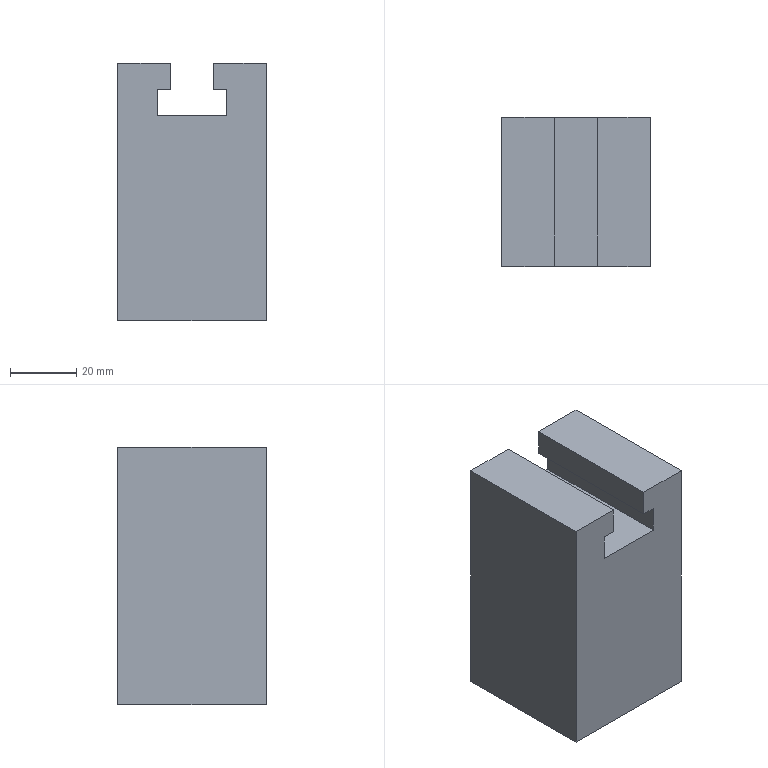Part | NX | features 模具.stp<1>[89] 2 | 1 solid | 22 faces | box 45 x 45 x 78 mm | volume 144302 mm3 | plane 18 | cylinder 3 | cone 1 | commonest cylinder face diameters 8.5 x1 9.7 x1 10 x1
STEP:
#1=CARTESIAN_POINT('',(-57.5,-211.5,-190.505));
#2=VERTEX_POINT('',#1);
#3=VERTEX_LOOP('',#2);
#4=FACE_BOUND('',#3,.T.);
#5=CARTESIAN_POINT('',(-57.5,-207.25,-192.959));
#6=VERTEX_POINT('',#5);
#7=CARTESIAN_POINT('',(-57.5,-211.5,-192.959));
#8=DIRECTION('',(0.,0.,-1.));
#9=DIRECTION('',(0.,1.,0.));
#10=AXIS2_PLACEMENT_3D('',#7,#8,#9);
#11=CIRCLE('',#10,4.25);
#12=EDGE_CURVE('',#6,#6,#11,.T.);
#13=ORIENTED_EDGE('',*,*,#12,.T.);
#14=EDGE_LOOP('',(#13));
#15=FACE_BOUND('',#14,.T.);
#16=CARTESIAN_POINT('',(-57.5,-211.5,-191.505));
#17=DIRECTION('',(0.,0.,-1.));
#18=DIRECTION('',(0.,1.,0.));
#19=AXIS2_PLACEMENT_3D('',#16,#17,#18);
#20=CONICAL_SURFACE('',#19,1.732,1.047);
#21=ADVANCED_FACE('',(#4,#15),#20,.F.);
#22=CARTESIAN_POINT('',(-57.5,-207.25,-196.5));
#23=VERTEX_POINT('',#22);
#24=CARTESIAN_POINT('',(-57.5,-206.65,-196.5));
#25=VERTEX_POINT('',#24);
#26=CARTESIAN_POINT('',(-57.5,-211.5,-196.5));
#27=DIRECTION('',(0.,1.,0.));
#28=VECTOR('',#27,1000.);
#29=LINE('',#26,#28);
#30=EDGE_CURVE('',#23,#25,#29,.T.);
#31=ORIENTED_EDGE('',*,*,#30,.T.);
#32=CARTESIAN_POINT('',(-52.65,-211.5,-196.5));
#33=VERTEX_POINT('',#32);
#34=CARTESIAN_POINT('',(-57.5,-211.5,-196.5));
#35=DIRECTION('',(0.,0.,1.));
#36=DIRECTION('',(0.,1.,0.));
#37=AXIS2_PLACEMENT_3D('',#34,#35,#36);
#38=CIRCLE('',#37,4.85);
#39=EDGE_CURVE('',#25,#33,#38,.T.);
#40=ORIENTED_EDGE('',*,*,#39,.T.);
#41=CARTESIAN_POINT('',(-53.25,-211.5,-196.5));
#42=VERTEX_POINT('',#41);
#43=CARTESIAN_POINT('',(-57.5,-211.5,-196.5));
#44=DIRECTION('',(-1.,0.,0.));
#45=VECTOR('',#44,1000.);
#46=LINE('',#43,#45);
#47=EDGE_CURVE('',#33,#42,#46,.T.);
#48=ORIENTED_EDGE('',*,*,#47,.T.);
#49=CARTESIAN_POINT('',(-57.5,-211.5,-196.5));
#50=DIRECTION('',(0.,0.,-1.));
#51=DIRECTION('',(1.,0.,0.));
#52=AXIS2_PLACEMENT_3D('',#49,#50,#51);
#53=CIRCLE('',#52,4.25);
#54=EDGE_CURVE('',#42,#23,#53,.T.);
#55=ORIENTED_EDGE('',*,*,#54,.T.);
#56=EDGE_LOOP('',(#31,#40,#48,#55));
#57=FACE_BOUND('',#56,.T.);
#58=CARTESIAN_POINT('',(-57.5,-211.5,-196.5));
#59=DIRECTION('',(0.,0.,1.));
#60=DIRECTION('',(1.,0.,0.));
#61=AXIS2_PLACEMENT_3D('',#58,#59,#60);
#62=PLANE('',#61);
#63=ADVANCED_FACE('',(#57),#62,.T.);
#64=CARTESIAN_POINT('',(-53.25,-211.5,-195.5));
#65=VERTEX_POINT('',#64);
#66=CARTESIAN_POINT('',(-57.5,-207.25,-195.5));
#67=VERTEX_POINT('',#66);
#68=CARTESIAN_POINT('',(-57.5,-211.5,-195.5));
#69=DIRECTION('',(0.,0.,-1.));
#70=DIRECTION('',(1.,0.,0.));
#71=AXIS2_PLACEMENT_3D('',#68,#69,#70);
#72=CIRCLE('',#71,4.25);
#73=EDGE_CURVE('',#65,#67,#72,.T.);
#74=ORIENTED_EDGE('',*,*,#73,.F.);
#75=CARTESIAN_POINT('',(-52.5,-211.5,-195.5));
#76=VERTEX_POINT('',#75);
#77=CARTESIAN_POINT('',(-52.5,-211.5,-195.5));
#78=DIRECTION('',(1.,0.,0.));
#79=VECTOR('',#78,1000.);
#80=LINE('',#77,#79);
#81=EDGE_CURVE('',#65,#76,#80,.T.);
#82=ORIENTED_EDGE('',*,*,#81,.T.);
#83=CARTESIAN_POINT('',(-57.5,-206.5,-195.5));
#84=VERTEX_POINT('',#83);
#85=CARTESIAN_POINT('',(-57.5,-211.5,-195.5));
#86=DIRECTION('',(0.,0.,1.));
#87=DIRECTION('',(0.,1.,0.));
#88=AXIS2_PLACEMENT_3D('',#85,#86,#87);
#89=CIRCLE('',#88,5.);
#90=EDGE_CURVE('',#84,#76,#89,.T.);
#91=ORIENTED_EDGE('',*,*,#90,.F.);
#92=CARTESIAN_POINT('',(-57.5,-206.5,-195.5));
#93=DIRECTION('',(0.,-1.,0.));
#94=VECTOR('',#93,1000.);
#95=LINE('',#92,#94);
#96=EDGE_CURVE('',#84,#67,#95,.T.);
#97=ORIENTED_EDGE('',*,*,#96,.T.);
#98=EDGE_LOOP('',(#74,#82,#91,#97));
#99=FACE_BOUND('',#98,.T.);
#100=CARTESIAN_POINT('',(-57.5,-211.5,-195.5));
#101=DIRECTION('',(0.,0.,1.));
#102=DIRECTION('',(1.,0.,0.));
#103=AXIS2_PLACEMENT_3D('',#100,#101,#102);
#104=PLANE('',#103);
#105=ADVANCED_FACE('',(#99),#104,.F.);
#106=CARTESIAN_POINT('',(-53.25,-211.5,-215.5));
#107=VERTEX_POINT('',#106);
#108=CARTESIAN_POINT('',(-57.5,-211.5,-215.5));
#109=DIRECTION('',(0.,0.,1.));
#110=DIRECTION('',(1.,0.,0.));
#111=AXIS2_PLACEMENT_3D('',#108,#109,#110);
#112=CIRCLE('',#111,4.25);
#113=EDGE_CURVE('',#107,#107,#112,.T.);
#114=ORIENTED_EDGE('',*,*,#113,.F.);
#115=EDGE_LOOP('',(#114));
#116=FACE_BOUND('',#115,.T.);
#117=ORIENTED_EDGE('',*,*,#12,.F.);
#118=EDGE_LOOP('',(#117));
#119=FACE_BOUND('',#118,.T.);
#120=CARTESIAN_POINT('',(-57.5,-207.25,-192.959));
#121=DIRECTION('',(0.,0.,1.));
#122=VECTOR('',#121,1000.);
#123=LINE('',#120,#122);
#124=EDGE_CURVE('',#23,#67,#123,.T.);
#125=ORIENTED_EDGE('',*,*,#124,.F.);
#126=ORIENTED_EDGE('',*,*,#54,.F.);
#127=CARTESIAN_POINT('',(-53.25,-211.5,-192.959));
#128=DIRECTION('',(0.,0.,-1.));
#129=VECTOR('',#128,1000.);
#130=LINE('',#127,#129);
#131=EDGE_CURVE('',#65,#42,#130,.T.);
#132=ORIENTED_EDGE('',*,*,#131,.F.);
#133=ORIENTED_EDGE('',*,*,#73,.T.);
#134=EDGE_LOOP('',(#125,#126,#132,#133));
#135=FACE_BOUND('',#134,.T.);
#136=CARTESIAN_POINT('',(-57.5,-211.5,-192.959));
#137=DIRECTION('',(0.,0.,-1.));
#138=DIRECTION('',(0.,1.,0.));
#139=AXIS2_PLACEMENT_3D('',#136,#137,#138);
#140=CYLINDRICAL_SURFACE('',#139,4.25);
#141=ADVANCED_FACE('',(#116,#119,#135),#140,.F.);
#142=CARTESIAN_POINT('',(-52.65,-211.5,-215.5));
#143=VERTEX_POINT('',#142);
#144=CARTESIAN_POINT('',(-52.5,-211.5,-215.5));
#145=VERTEX_POINT('',#144);
#146=CARTESIAN_POINT('',(-82.5,-211.5,-215.5));
#147=DIRECTION('',(1.,0.,0.));
#148=VECTOR('',#147,1000.);
#149=LINE('',#146,#148);
#150=EDGE_CURVE('',#143,#145,#149,.T.);
#151=ORIENTED_EDGE('',*,*,#150,.T.);
#152=CARTESIAN_POINT('',(-52.5,-211.5,-195.5));
#153=DIRECTION('',(0.,0.,1.));
#154=VECTOR('',#153,1000.);
#155=LINE('',#152,#154);
#156=EDGE_CURVE('',#145,#76,#155,.T.);
#157=ORIENTED_EDGE('',*,*,#156,.T.);
#158=ORIENTED_EDGE('',*,*,#81,.F.);
#159=ORIENTED_EDGE('',*,*,#131,.T.);
#160=ORIENTED_EDGE('',*,*,#47,.F.);
#161=CARTESIAN_POINT('',(-52.65,-211.5,-196.5));
#162=DIRECTION('',(0.,0.,1.));
#163=VECTOR('',#162,1000.);
#164=LINE('',#161,#163);
#165=EDGE_CURVE('',#143,#33,#164,.T.);
#166=ORIENTED_EDGE('',*,*,#165,.F.);
#167=EDGE_LOOP('',(#151,#157,#158,#159,#160,#166));
#168=FACE_BOUND('',#167,.T.);
#169=CARTESIAN_POINT('',(-52.5,-211.5,-195.5));
#170=DIRECTION('',(0.,-1.,0.));
#171=DIRECTION('',(0.,0.,-1.));
#172=AXIS2_PLACEMENT_3D('',#169,#170,#171);
#173=PLANE('',#172);
#174=ADVANCED_FACE('',(#168),#173,.T.);
#175=CARTESIAN_POINT('',(-57.5,-206.5,-215.5));
#176=VERTEX_POINT('',#175);
#177=CARTESIAN_POINT('',(-57.5,-206.65,-215.5));
#178=VERTEX_POINT('',#177);
#179=CARTESIAN_POINT('',(-57.5,-245.,-215.5));
#180=DIRECTION('',(0.,-1.,0.));
#181=VECTOR('',#180,1000.);
#182=LINE('',#179,#181);
#183=EDGE_CURVE('',#176,#178,#182,.T.);
#184=ORIENTED_EDGE('',*,*,#183,.T.);
#185=CARTESIAN_POINT('',(-57.5,-206.65,-196.5));
#186=DIRECTION('',(0.,0.,-1.));
#187=VECTOR('',#186,1000.);
#188=LINE('',#185,#187);
#189=EDGE_CURVE('',#25,#178,#188,.T.);
#190=ORIENTED_EDGE('',*,*,#189,.F.);
#191=ORIENTED_EDGE('',*,*,#30,.F.);
#192=ORIENTED_EDGE('',*,*,#124,.T.);
#193=ORIENTED_EDGE('',*,*,#96,.F.);
#194=CARTESIAN_POINT('',(-57.5,-206.5,-195.5));
#195=DIRECTION('',(0.,0.,-1.));
#196=VECTOR('',#195,1000.);
#197=LINE('',#194,#196);
#198=EDGE_CURVE('',#84,#176,#197,.T.);
#199=ORIENTED_EDGE('',*,*,#198,.T.);
#200=EDGE_LOOP('',(#184,#190,#191,#192,#193,#199));
#201=FACE_BOUND('',#200,.T.);
#202=CARTESIAN_POINT('',(-57.5,-206.5,-195.5));
#203=DIRECTION('',(-1.,0.,0.));
#204=DIRECTION('',(0.,1.,0.));
#205=AXIS2_PLACEMENT_3D('',#202,#203,#204);
#206=PLANE('',#205);
#207=ADVANCED_FACE('',(#201),#206,.T.);
#208=CARTESIAN_POINT('',(-57.5,-211.5,-215.5));
#209=DIRECTION('',(0.,0.,1.));
#210=DIRECTION('',(1.,0.,0.));
#211=AXIS2_PLACEMENT_3D('',#208,#209,#210);
#212=CIRCLE('',#211,4.85);
#213=EDGE_CURVE('',#178,#143,#212,.T.);
#214=ORIENTED_EDGE('',*,*,#213,.T.);
#215=ORIENTED_EDGE('',*,*,#165,.T.);
#216=ORIENTED_EDGE('',*,*,#39,.F.);
#217=ORIENTED_EDGE('',*,*,#189,.T.);
#218=EDGE_LOOP('',(#214,#215,#216,#217));
#219=FACE_BOUND('',#218,.T.);
#220=CARTESIAN_POINT('',(-57.5,-211.5,-196.5));
#221=DIRECTION('',(0.,0.,-1.));
#222=DIRECTION('',(0.,1.,0.));
#223=AXIS2_PLACEMENT_3D('',#220,#221,#222);
#224=CYLINDRICAL_SURFACE('',#223,4.85);
#225=ADVANCED_FACE('',(#219),#224,.T.);
#226=ORIENTED_EDGE('',*,*,#198,.F.);
#227=ORIENTED_EDGE('',*,*,#90,.T.);
#228=ORIENTED_EDGE('',*,*,#156,.F.);
#229=CARTESIAN_POINT('',(-57.5,-211.5,-215.5));
#230=DIRECTION('',(0.,0.,1.));
#231=DIRECTION('',(1.,0.,0.));
#232=AXIS2_PLACEMENT_3D('',#229,#230,#231);
#233=CIRCLE('',#232,5.);
#234=EDGE_CURVE('',#176,#145,#233,.T.);
#235=ORIENTED_EDGE('',*,*,#234,.F.);
#236=EDGE_LOOP('',(#226,#227,#228,#235));
#237=FACE_BOUND('',#236,.T.);
#238=CARTESIAN_POINT('',(-57.5,-211.5,-195.5));
#239=DIRECTION('',(0.,0.,-1.));
#240=DIRECTION('',(0.,1.,0.));
#241=AXIS2_PLACEMENT_3D('',#238,#239,#240);
#242=CYLINDRICAL_SURFACE('',#241,5.);
#243=ADVANCED_FACE('',(#237),#242,.F.);
#244=CARTESIAN_POINT('',(-64.,-234.,-145.5));
#245=VERTEX_POINT('',#244);
#246=CARTESIAN_POINT('',(-68.,-234.,-145.5));
#247=VERTEX_POINT('',#246);
#248=CARTESIAN_POINT('',(-67.5,-234.,-145.5));
#249=DIRECTION('',(-1.,0.,0.));
#250=VECTOR('',#249,1000.);
#251=LINE('',#248,#250);
#252=EDGE_CURVE('',#245,#247,#251,.T.);
#253=ORIENTED_EDGE('',*,*,#252,.T.);
#254=CARTESIAN_POINT('',(-68.,-189.,-145.5));
#255=VERTEX_POINT('',#254);
#256=CARTESIAN_POINT('',(-68.,-197.846,-145.5));
#257=DIRECTION('',(0.,-1.,0.));
#258=VECTOR('',#257,1000.);
#259=LINE('',#256,#258);
#260=EDGE_CURVE('',#255,#247,#259,.T.);
#261=ORIENTED_EDGE('',*,*,#260,.F.);
#262=CARTESIAN_POINT('',(-64.,-189.,-145.5));
#263=VERTEX_POINT('',#262);
#264=CARTESIAN_POINT('',(-67.5,-189.,-145.5));
#265=DIRECTION('',(1.,0.,0.));
#266=VECTOR('',#265,1000.);
#267=LINE('',#264,#266);
#268=EDGE_CURVE('',#255,#263,#267,.T.);
#269=ORIENTED_EDGE('',*,*,#268,.T.);
#270=CARTESIAN_POINT('',(-64.,-264.,-145.5));
#271=DIRECTION('',(0.,1.,0.));
#272=VECTOR('',#271,1000.);
#273=LINE('',#270,#272);
#274=EDGE_CURVE('',#245,#263,#273,.T.);
#275=ORIENTED_EDGE('',*,*,#274,.F.);
#276=EDGE_LOOP('',(#253,#261,#269,#275));
#277=FACE_BOUND('',#276,.T.);
#278=CARTESIAN_POINT('',(-67.5,-264.,-145.5));
#279=DIRECTION('',(0.,0.,1.));
#280=DIRECTION('',(1.,0.,0.));
#281=AXIS2_PLACEMENT_3D('',#278,#279,#280);
#282=PLANE('',#281);
#283=ADVANCED_FACE('',(#277),#282,.F.);
#284=CARTESIAN_POINT('',(-47.,-234.,-145.5));
#285=VERTEX_POINT('',#284);
#286=CARTESIAN_POINT('',(-51.,-234.,-145.5));
#287=VERTEX_POINT('',#286);
#288=CARTESIAN_POINT('',(-47.5,-234.,-145.5));
#289=DIRECTION('',(-1.,0.,0.));
#290=VECTOR('',#289,1000.);
#291=LINE('',#288,#290);
#292=EDGE_CURVE('',#285,#287,#291,.T.);
#293=ORIENTED_EDGE('',*,*,#292,.T.);
#294=CARTESIAN_POINT('',(-51.,-189.,-145.5));
#295=VERTEX_POINT('',#294);
#296=CARTESIAN_POINT('',(-51.,-264.,-145.5));
#297=DIRECTION('',(0.,-1.,0.));
#298=VECTOR('',#297,1000.);
#299=LINE('',#296,#298);
#300=EDGE_CURVE('',#295,#287,#299,.T.);
#301=ORIENTED_EDGE('',*,*,#300,.F.);
#302=CARTESIAN_POINT('',(-47.,-189.,-145.5));
#303=VERTEX_POINT('',#302);
#304=CARTESIAN_POINT('',(-47.5,-189.,-145.5));
#305=DIRECTION('',(1.,0.,0.));
#306=VECTOR('',#305,1000.);
#307=LINE('',#304,#306);
#308=EDGE_CURVE('',#295,#303,#307,.T.);
#309=ORIENTED_EDGE('',*,*,#308,.T.);
#310=CARTESIAN_POINT('',(-47.,-264.,-145.5));
#311=DIRECTION('',(0.,1.,0.));
#312=VECTOR('',#311,1000.);
#313=LINE('',#310,#312);
#314=EDGE_CURVE('',#285,#303,#313,.T.);
#315=ORIENTED_EDGE('',*,*,#314,.F.);
#316=EDGE_LOOP('',(#293,#301,#309,#315));
#317=FACE_BOUND('',#316,.T.);
#318=CARTESIAN_POINT('',(-47.5,-264.,-145.5));
#319=DIRECTION('',(0.,0.,1.));
#320=DIRECTION('',(1.,0.,0.));
#321=AXIS2_PLACEMENT_3D('',#318,#319,#320);
#322=PLANE('',#321);
#323=ADVANCED_FACE('',(#317),#322,.F.);
#324=CARTESIAN_POINT('',(-68.,-234.,-153.5));
#325=VERTEX_POINT('',#324);
#326=CARTESIAN_POINT('',(-68.,-234.,0.));
#327=DIRECTION('',(0.,0.,1.));
#328=VECTOR('',#327,1000.);
#329=LINE('',#326,#328);
#330=EDGE_CURVE('',#325,#247,#329,.T.);
#331=ORIENTED_EDGE('',*,*,#330,.F.);
#332=CARTESIAN_POINT('',(-68.,-189.,-153.5));
#333=VERTEX_POINT('',#332);
#334=CARTESIAN_POINT('',(-68.,-197.846,-153.5));
#335=DIRECTION('',(0.,-1.,0.));
#336=VECTOR('',#335,1000.);
#337=LINE('',#334,#336);
#338=EDGE_CURVE('',#333,#325,#337,.T.);
#339=ORIENTED_EDGE('',*,*,#338,.F.);
#340=CARTESIAN_POINT('',(-68.,-189.,19.75));
#341=DIRECTION('',(0.,0.,-1.));
#342=VECTOR('',#341,1000.);
#343=LINE('',#340,#342);
#344=EDGE_CURVE('',#255,#333,#343,.T.);
#345=ORIENTED_EDGE('',*,*,#344,.F.);
#346=ORIENTED_EDGE('',*,*,#260,.T.);
#347=EDGE_LOOP('',(#331,#339,#345,#346));
#348=FACE_BOUND('',#347,.T.);
#349=CARTESIAN_POINT('',(-68.,-197.846,19.75));
#350=DIRECTION('',(1.,0.,0.));
#351=DIRECTION('',(0.,0.,-1.));
#352=AXIS2_PLACEMENT_3D('',#349,#350,#351);
#353=PLANE('',#352);
#354=ADVANCED_FACE('',(#348),#353,.T.);
#355=ORIENTED_EDGE('',*,*,#338,.T.);
#356=CARTESIAN_POINT('',(-47.,-234.,-153.5));
#357=VERTEX_POINT('',#356);
#358=CARTESIAN_POINT('',(0.,-234.,-153.5));
#359=DIRECTION('',(1.,0.,0.));
#360=VECTOR('',#359,1000.);
#361=LINE('',#358,#360);
#362=EDGE_CURVE('',#325,#357,#361,.T.);
#363=ORIENTED_EDGE('',*,*,#362,.T.);
#364=CARTESIAN_POINT('',(-47.,-189.,-153.5));
#365=VERTEX_POINT('',#364);
#366=CARTESIAN_POINT('',(-47.,-197.846,-153.5));
#367=DIRECTION('',(0.,-1.,0.));
#368=VECTOR('',#367,1000.);
#369=LINE('',#366,#368);
#370=EDGE_CURVE('',#365,#357,#369,.T.);
#371=ORIENTED_EDGE('',*,*,#370,.F.);
#372=CARTESIAN_POINT('',(-32.5,-189.,-153.5));
#373=DIRECTION('',(1.,0.,0.));
#374=VECTOR('',#373,1000.);
#375=LINE('',#372,#374);
#376=EDGE_CURVE('',#333,#365,#375,.T.);
#377=ORIENTED_EDGE('',*,*,#376,.F.);
#378=EDGE_LOOP('',(#355,#363,#371,#377));
#379=FACE_BOUND('',#378,.T.);
#380=CARTESIAN_POINT('',(-32.5,-245.,-153.5));
#381=DIRECTION('',(0.,0.,-1.));
#382=DIRECTION('',(0.,-1.,0.));
#383=AXIS2_PLACEMENT_3D('',#380,#381,#382);
#384=PLANE('',#383);
#385=ADVANCED_FACE('',(#379),#384,.F.);
#386=CARTESIAN_POINT('',(-47.,-189.,19.75));
#387=DIRECTION('',(0.,0.,-1.));
#388=VECTOR('',#387,1000.);
#389=LINE('',#386,#388);
#390=EDGE_CURVE('',#303,#365,#389,.T.);
#391=ORIENTED_EDGE('',*,*,#390,.T.);
#392=ORIENTED_EDGE('',*,*,#370,.T.);
#393=CARTESIAN_POINT('',(-47.,-234.,0.));
#394=DIRECTION('',(0.,0.,1.));
#395=VECTOR('',#394,1000.);
#396=LINE('',#393,#395);
#397=EDGE_CURVE('',#357,#285,#396,.T.);
#398=ORIENTED_EDGE('',*,*,#397,.T.);
#399=ORIENTED_EDGE('',*,*,#314,.T.);
#400=EDGE_LOOP('',(#391,#392,#398,#399));
#401=FACE_BOUND('',#400,.T.);
#402=CARTESIAN_POINT('',(-47.,-197.846,19.75));
#403=DIRECTION('',(-1.,0.,0.));
#404=DIRECTION('',(0.,1.,0.));
#405=AXIS2_PLACEMENT_3D('',#402,#403,#404);
#406=PLANE('',#405);
#407=ADVANCED_FACE('',(#401),#406,.T.);
#408=CARTESIAN_POINT('',(-64.,-234.,-137.5));
#409=VERTEX_POINT('',#408);
#410=CARTESIAN_POINT('',(-64.,-234.,0.));
#411=DIRECTION('',(0.,0.,-1.));
#412=VECTOR('',#411,1000.);
#413=LINE('',#410,#412);
#414=EDGE_CURVE('',#409,#245,#413,.T.);
#415=ORIENTED_EDGE('',*,*,#414,.T.);
#416=ORIENTED_EDGE('',*,*,#274,.T.);
#417=CARTESIAN_POINT('',(-64.,-189.,-137.5));
#418=VERTEX_POINT('',#417);
#419=CARTESIAN_POINT('',(-64.,-189.,-145.5));
#420=DIRECTION('',(0.,0.,1.));
#421=VECTOR('',#420,1000.);
#422=LINE('',#419,#421);
#423=EDGE_CURVE('',#263,#418,#422,.T.);
#424=ORIENTED_EDGE('',*,*,#423,.T.);
#425=CARTESIAN_POINT('',(-64.,-245.,-137.5));
#426=DIRECTION('',(0.,1.,0.));
#427=VECTOR('',#426,1000.);
#428=LINE('',#425,#427);
#429=EDGE_CURVE('',#409,#418,#428,.T.);
#430=ORIENTED_EDGE('',*,*,#429,.F.);
#431=EDGE_LOOP('',(#415,#416,#424,#430));
#432=FACE_BOUND('',#431,.T.);
#433=CARTESIAN_POINT('',(-64.,-264.,-145.5));
#434=DIRECTION('',(-1.,0.,0.));
#435=DIRECTION('',(0.,0.,1.));
#436=AXIS2_PLACEMENT_3D('',#433,#434,#435);
#437=PLANE('',#436);
#438=ADVANCED_FACE('',(#432),#437,.F.);
#439=CARTESIAN_POINT('',(-51.,-189.,-137.5));
#440=VERTEX_POINT('',#439);
#441=CARTESIAN_POINT('',(-51.,-189.,-145.5));
#442=DIRECTION('',(0.,0.,-1.));
#443=VECTOR('',#442,1000.);
#444=LINE('',#441,#443);
#445=EDGE_CURVE('',#440,#295,#444,.T.);
#446=ORIENTED_EDGE('',*,*,#445,.T.);
#447=ORIENTED_EDGE('',*,*,#300,.T.);
#448=CARTESIAN_POINT('',(-51.,-234.,-137.5));
#449=VERTEX_POINT('',#448);
#450=CARTESIAN_POINT('',(-51.,-234.,0.));
#451=DIRECTION('',(0.,0.,1.));
#452=VECTOR('',#451,1000.);
#453=LINE('',#450,#452);
#454=EDGE_CURVE('',#287,#449,#453,.T.);
#455=ORIENTED_EDGE('',*,*,#454,.T.);
#456=CARTESIAN_POINT('',(-51.,-245.,-137.5));
#457=DIRECTION('',(0.,-1.,0.));
#458=VECTOR('',#457,1000.);
#459=LINE('',#456,#458);
#460=EDGE_CURVE('',#440,#449,#459,.T.);
#461=ORIENTED_EDGE('',*,*,#460,.F.);
#462=EDGE_LOOP('',(#446,#447,#455,#461));
#463=FACE_BOUND('',#462,.T.);
#464=CARTESIAN_POINT('',(-51.,-264.,-145.5));
#465=DIRECTION('',(1.,0.,0.));
#466=DIRECTION('',(0.,0.,-1.));
#467=AXIS2_PLACEMENT_3D('',#464,#465,#466);
#468=PLANE('',#467);
#469=ADVANCED_FACE('',(#463),#468,.F.);
#470=ORIENTED_EDGE('',*,*,#252,.F.);
#471=ORIENTED_EDGE('',*,*,#414,.F.);
#472=CARTESIAN_POINT('',(-80.,-234.,-137.5));
#473=VERTEX_POINT('',#472);
#474=CARTESIAN_POINT('',(-32.5,-234.,-137.5));
#475=DIRECTION('',(-1.,0.,0.));
#476=VECTOR('',#475,1000.);
#477=LINE('',#474,#476);
#478=EDGE_CURVE('',#409,#473,#477,.T.);
#479=ORIENTED_EDGE('',*,*,#478,.T.);
#480=CARTESIAN_POINT('',(-80.,-234.,-215.5));
#481=VERTEX_POINT('',#480);
#482=CARTESIAN_POINT('',(-80.,-234.,-137.5));
#483=DIRECTION('',(0.,0.,-1.));
#484=VECTOR('',#483,1000.);
#485=LINE('',#482,#484);
#486=EDGE_CURVE('',#473,#481,#485,.T.);
#487=ORIENTED_EDGE('',*,*,#486,.T.);
#488=CARTESIAN_POINT('',(-35.,-234.,-215.5));
#489=VERTEX_POINT('',#488);
#490=CARTESIAN_POINT('',(-82.5,-234.,-215.5));
#491=DIRECTION('',(1.,0.,0.));
#492=VECTOR('',#491,1000.);
#493=LINE('',#490,#492);
#494=EDGE_CURVE('',#481,#489,#493,.T.);
#495=ORIENTED_EDGE('',*,*,#494,.T.);
#496=CARTESIAN_POINT('',(-35.,-234.,-137.5));
#497=VERTEX_POINT('',#496);
#498=CARTESIAN_POINT('',(-35.,-234.,-215.5));
#499=DIRECTION('',(0.,0.,1.));
#500=VECTOR('',#499,1000.);
#501=LINE('',#498,#500);
#502=EDGE_CURVE('',#489,#497,#501,.T.);
#503=ORIENTED_EDGE('',*,*,#502,.T.);
#504=CARTESIAN_POINT('',(-32.5,-234.,-137.5));
#505=DIRECTION('',(-1.,0.,0.));
#506=VECTOR('',#505,1000.);
#507=LINE('',#504,#506);
#508=EDGE_CURVE('',#497,#449,#507,.T.);
#509=ORIENTED_EDGE('',*,*,#508,.T.);
#510=ORIENTED_EDGE('',*,*,#454,.F.);
#511=ORIENTED_EDGE('',*,*,#292,.F.);
#512=ORIENTED_EDGE('',*,*,#397,.F.);
#513=ORIENTED_EDGE('',*,*,#362,.F.);
#514=ORIENTED_EDGE('',*,*,#330,.T.);
#515=EDGE_LOOP('',(#470,#471,#479,#487,#495,#503,#509,#510,#511,#512,#513,#514));
#516=FACE_BOUND('',#515,.T.);
#517=CARTESIAN_POINT('',(0.,-234.,0.));
#518=DIRECTION('',(0.,-1.,0.));
#519=DIRECTION('',(0.,0.,-1.));
#520=AXIS2_PLACEMENT_3D('',#517,#518,#519);
#521=PLANE('',#520);
#522=ADVANCED_FACE('',(#516),#521,.T.);
#523=ORIENTED_EDGE('',*,*,#429,.T.);
#524=CARTESIAN_POINT('',(-80.,-189.,-137.5));
#525=VERTEX_POINT('',#524);
#526=CARTESIAN_POINT('',(-32.5,-189.,-137.5));
#527=DIRECTION('',(-1.,0.,0.));
#528=VECTOR('',#527,1000.);
#529=LINE('',#526,#528);
#530=EDGE_CURVE('',#418,#525,#529,.T.);
#531=ORIENTED_EDGE('',*,*,#530,.T.);
#532=CARTESIAN_POINT('',(-80.,-245.,-137.5));
#533=DIRECTION('',(0.,1.,0.));
#534=VECTOR('',#533,1000.);
#535=LINE('',#532,#534);
#536=EDGE_CURVE('',#473,#525,#535,.T.);
#537=ORIENTED_EDGE('',*,*,#536,.F.);
#538=ORIENTED_EDGE('',*,*,#478,.F.);
#539=EDGE_LOOP('',(#523,#531,#537,#538));
#540=FACE_BOUND('',#539,.T.);
#541=CARTESIAN_POINT('',(-32.5,-245.,-137.5));
#542=DIRECTION('',(0.,0.,-1.));
#543=DIRECTION('',(0.,-1.,0.));
#544=AXIS2_PLACEMENT_3D('',#541,#542,#543);
#545=PLANE('',#544);
#546=ADVANCED_FACE('',(#540),#545,.F.);
#547=CARTESIAN_POINT('',(-35.,-189.,-215.5));
#548=VERTEX_POINT('',#547);
#549=CARTESIAN_POINT('',(-35.,-189.,-137.5));
#550=VERTEX_POINT('',#549);
#551=CARTESIAN_POINT('',(-35.,-189.,-215.5));
#552=DIRECTION('',(0.,0.,1.));
#553=VECTOR('',#552,1000.);
#554=LINE('',#551,#553);
#555=EDGE_CURVE('',#548,#550,#554,.T.);
#556=ORIENTED_EDGE('',*,*,#555,.T.);
#557=CARTESIAN_POINT('',(-35.,-245.,-137.5));
#558=DIRECTION('',(0.,1.,0.));
#559=VECTOR('',#558,1000.);
#560=LINE('',#557,#559);
#561=EDGE_CURVE('',#497,#550,#560,.T.);
#562=ORIENTED_EDGE('',*,*,#561,.F.);
#563=ORIENTED_EDGE('',*,*,#502,.F.);
#564=CARTESIAN_POINT('',(-35.,-245.,-215.5));
#565=DIRECTION('',(0.,1.,0.));
#566=VECTOR('',#565,1000.);
#567=LINE('',#564,#566);
#568=EDGE_CURVE('',#489,#548,#567,.T.);
#569=ORIENTED_EDGE('',*,*,#568,.T.);
#570=EDGE_LOOP('',(#556,#562,#563,#569));
#571=FACE_BOUND('',#570,.T.);
#572=CARTESIAN_POINT('',(-35.,-245.,-215.5));
#573=DIRECTION('',(-1.,0.,0.));
#574=DIRECTION('',(0.,1.,0.));
#575=AXIS2_PLACEMENT_3D('',#572,#573,#574);
#576=PLANE('',#575);
#577=ADVANCED_FACE('',(#571),#576,.F.);
#578=CARTESIAN_POINT('',(-80.,-189.,-215.5));
#579=VERTEX_POINT('',#578);
#580=CARTESIAN_POINT('',(-80.,-189.,-137.5));
#581=DIRECTION('',(0.,0.,-1.));
#582=VECTOR('',#581,1000.);
#583=LINE('',#580,#582);
#584=EDGE_CURVE('',#525,#579,#583,.T.);
#585=ORIENTED_EDGE('',*,*,#584,.T.);
#586=CARTESIAN_POINT('',(-80.,-245.,-215.5));
#587=DIRECTION('',(0.,1.,0.));
#588=VECTOR('',#587,1000.);
#589=LINE('',#586,#588);
#590=EDGE_CURVE('',#481,#579,#589,.T.);
#591=ORIENTED_EDGE('',*,*,#590,.F.);
#592=ORIENTED_EDGE('',*,*,#486,.F.);
#593=ORIENTED_EDGE('',*,*,#536,.T.);
#594=EDGE_LOOP('',(#585,#591,#592,#593));
#595=FACE_BOUND('',#594,.T.);
#596=CARTESIAN_POINT('',(-80.,-245.,-137.5));
#597=DIRECTION('',(1.,0.,0.));
#598=DIRECTION('',(0.,0.,1.));
#599=AXIS2_PLACEMENT_3D('',#596,#597,#598);
#600=PLANE('',#599);
#601=ADVANCED_FACE('',(#595),#600,.F.);
#602=CARTESIAN_POINT('',(-32.5,-189.,-137.5));
#603=DIRECTION('',(-1.,0.,0.));
#604=VECTOR('',#603,1000.);
#605=LINE('',#602,#604);
#606=EDGE_CURVE('',#550,#440,#605,.T.);
#607=ORIENTED_EDGE('',*,*,#606,.T.);
#608=ORIENTED_EDGE('',*,*,#460,.T.);
#609=ORIENTED_EDGE('',*,*,#508,.F.);
#610=ORIENTED_EDGE('',*,*,#561,.T.);
#611=EDGE_LOOP('',(#607,#608,#609,#610));
#612=FACE_BOUND('',#611,.T.);
#613=CARTESIAN_POINT('',(-32.5,-245.,-137.5));
#614=DIRECTION('',(0.,0.,-1.));
#615=DIRECTION('',(0.,-1.,0.));
#616=AXIS2_PLACEMENT_3D('',#613,#614,#615);
#617=PLANE('',#616);
#618=ADVANCED_FACE('',(#612),#617,.F.);
#619=ORIENTED_EDGE('',*,*,#445,.F.);
#620=ORIENTED_EDGE('',*,*,#606,.F.);
#621=ORIENTED_EDGE('',*,*,#555,.F.);
#622=CARTESIAN_POINT('',(-82.5,-189.,-215.5));
#623=DIRECTION('',(1.,0.,0.));
#624=VECTOR('',#623,1000.);
#625=LINE('',#622,#624);
#626=EDGE_CURVE('',#579,#548,#625,.T.);
#627=ORIENTED_EDGE('',*,*,#626,.F.);
#628=ORIENTED_EDGE('',*,*,#584,.F.);
#629=ORIENTED_EDGE('',*,*,#530,.F.);
#630=ORIENTED_EDGE('',*,*,#423,.F.);
#631=ORIENTED_EDGE('',*,*,#268,.F.);
#632=ORIENTED_EDGE('',*,*,#344,.T.);
#633=ORIENTED_EDGE('',*,*,#376,.T.);
#634=ORIENTED_EDGE('',*,*,#390,.F.);
#635=ORIENTED_EDGE('',*,*,#308,.F.);
#636=EDGE_LOOP('',(#619,#620,#621,#627,#628,#629,#630,#631,#632,#633,#634,#635));
#637=FACE_BOUND('',#636,.T.);
#638=CARTESIAN_POINT('',(0.,-189.,0.));
#639=DIRECTION('',(0.,-1.,0.));
#640=DIRECTION('',(0.,0.,-1.));
#641=AXIS2_PLACEMENT_3D('',#638,#639,#640);
#642=PLANE('',#641);
#643=ADVANCED_FACE('',(#637),#642,.F.);
#644=ORIENTED_EDGE('',*,*,#183,.F.);
#645=ORIENTED_EDGE('',*,*,#234,.T.);
#646=ORIENTED_EDGE('',*,*,#150,.F.);
#647=ORIENTED_EDGE('',*,*,#213,.F.);
#648=EDGE_LOOP('',(#644,#645,#646,#647));
#649=FACE_BOUND('',#648,.T.);
#650=ORIENTED_EDGE('',*,*,#113,.T.);
#651=EDGE_LOOP('',(#650));
#652=FACE_BOUND('',#651,.T.);
#653=ORIENTED_EDGE('',*,*,#626,.T.);
#654=ORIENTED_EDGE('',*,*,#568,.F.);
#655=ORIENTED_EDGE('',*,*,#494,.F.);
#656=ORIENTED_EDGE('',*,*,#590,.T.);
#657=EDGE_LOOP('',(#653,#654,#655,#656));
#658=FACE_BOUND('',#657,.T.);
#659=CARTESIAN_POINT('',(-82.5,-245.,-215.5));
#660=DIRECTION('',(0.,0.,1.));
#661=DIRECTION('',(1.,0.,0.));
#662=AXIS2_PLACEMENT_3D('',#659,#660,#661);
#663=PLANE('',#662);
#664=ADVANCED_FACE('',(#649,#652,#658),#663,.F.);
#665=CLOSED_SHELL('',(#21,#63,#105,#141,#174,#207,#225,#243,#283,#323,#354,#385,#407,#438,#469,#522,#546,#577,#601,#618,#643,#664));
#666=MANIFOLD_SOLID_BREP('',#665);
#667=(LENGTH_UNIT()NAMED_UNIT(*)SI_UNIT(.MILLI.,.METRE.));
#668=UNCERTAINTY_MEASURE_WITH_UNIT(LENGTH_MEASURE(0.00001),#667,'','');
#669=(NAMED_UNIT(*)PLANE_ANGLE_UNIT()SI_UNIT($,.RADIAN.));
#670=(NAMED_UNIT(*)SI_UNIT($,.STERADIAN.)SOLID_ANGLE_UNIT());
#671=(GEOMETRIC_REPRESENTATION_CONTEXT(3)GLOBAL_UNCERTAINTY_ASSIGNED_CONTEXT((#668))GLOBAL_UNIT_ASSIGNED_CONTEXT((#667,#669,#670))REPRESENTATION_CONTEXT('',''));
#672=ADVANCED_BREP_SHAPE_REPRESENTATION('',(#666),#671);